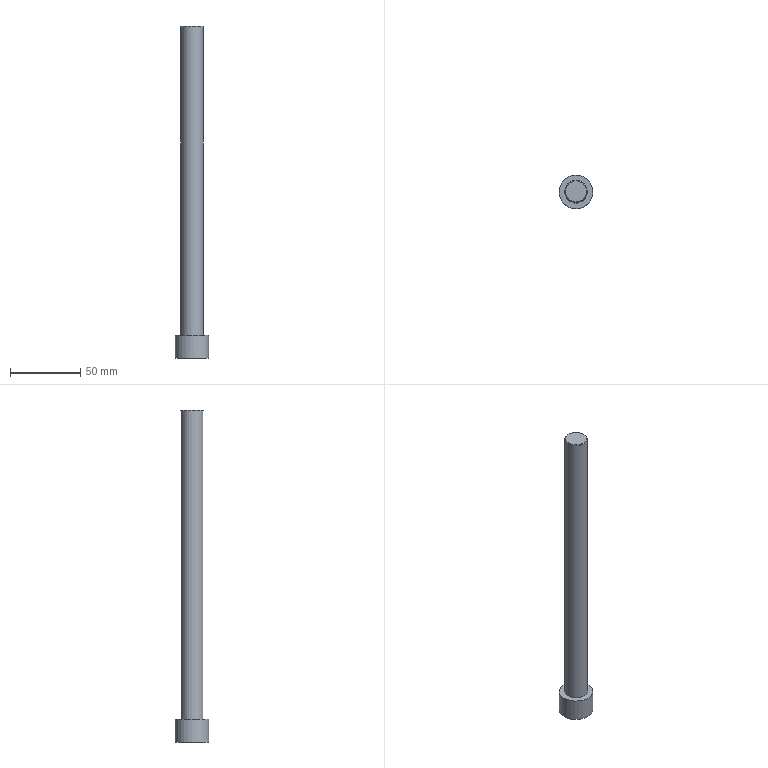Part | STEP file | 1_id586_xmt_txt | 1 solid | 19 faces | box 24 x 24 x 236 mm | volume 50039 mm3 | plane 15 | cylinder 2 | cone 2 | commonest cylinder face diameters 16 x1 24 x1
STEP:
#1=CARTESIAN_POINT('',(-153.,262.,-278.));
#2=VERTEX_POINT('',#1);
#3=CARTESIAN_POINT('',(-165.,262.,-278.));
#4=DIRECTION('',(0.,0.,-1.));
#5=DIRECTION('',(1.,0.,0.));
#6=AXIS2_PLACEMENT_3D('',#3,#4,#5);
#7=CIRCLE('',#6,12.);
#8=EDGE_CURVE('',#2,#2,#7,.T.);
#9=ORIENTED_EDGE('',*,*,#8,.F.);
#10=EDGE_LOOP('',(#9));
#11=FACE_BOUND('',#10,.T.);
#12=CARTESIAN_POINT('',(-153.,262.,-262.));
#13=VERTEX_POINT('',#12);
#14=CARTESIAN_POINT('',(-165.,262.,-262.));
#15=DIRECTION('',(0.,0.,1.));
#16=DIRECTION('',(1.,0.,0.));
#17=AXIS2_PLACEMENT_3D('',#14,#15,#16);
#18=CIRCLE('',#17,12.);
#19=EDGE_CURVE('',#13,#13,#18,.T.);
#20=ORIENTED_EDGE('',*,*,#19,.F.);
#21=EDGE_LOOP('',(#20));
#22=FACE_BOUND('',#21,.T.);
#23=CARTESIAN_POINT('',(-165.,262.,-270.));
#24=DIRECTION('',(0.,0.,1.));
#25=DIRECTION('',(-1.,0.,0.));
#26=AXIS2_PLACEMENT_3D('',#23,#24,#25);
#27=CYLINDRICAL_SURFACE('',#26,12.);
#28=ADVANCED_FACE('',(#11,#22),#27,.T.);
#29=CARTESIAN_POINT('',(-165.,270.083,-270.));
#30=VERTEX_POINT('',#29);
#31=CARTESIAN_POINT('',(-158.,266.041,-270.));
#32=VERTEX_POINT('',#31);
#33=CARTESIAN_POINT('',(-165.,262.,-270.));
#34=DIRECTION('',(0.,0.,-1.));
#35=DIRECTION('',(1.,0.,0.));
#36=AXIS2_PLACEMENT_3D('',#33,#34,#35);
#37=CIRCLE('',#36,8.083);
#38=EDGE_CURVE('',#30,#32,#37,.T.);
#39=ORIENTED_EDGE('',*,*,#38,.T.);
#40=CARTESIAN_POINT('',(-158.,257.959,-270.));
#41=VERTEX_POINT('',#40);
#42=CARTESIAN_POINT('',(-165.,262.,-270.));
#43=DIRECTION('',(0.,0.,-1.));
#44=DIRECTION('',(1.,0.,0.));
#45=AXIS2_PLACEMENT_3D('',#42,#43,#44);
#46=CIRCLE('',#45,8.083);
#47=EDGE_CURVE('',#32,#41,#46,.T.);
#48=ORIENTED_EDGE('',*,*,#47,.T.);
#49=CARTESIAN_POINT('',(-165.,253.917,-270.));
#50=VERTEX_POINT('',#49);
#51=CARTESIAN_POINT('',(-165.,262.,-270.));
#52=DIRECTION('',(0.,0.,-1.));
#53=DIRECTION('',(1.,0.,0.));
#54=AXIS2_PLACEMENT_3D('',#51,#52,#53);
#55=CIRCLE('',#54,8.083);
#56=EDGE_CURVE('',#41,#50,#55,.T.);
#57=ORIENTED_EDGE('',*,*,#56,.T.);
#58=CARTESIAN_POINT('',(-172.,257.959,-270.));
#59=VERTEX_POINT('',#58);
#60=CARTESIAN_POINT('',(-165.,262.,-270.));
#61=DIRECTION('',(0.,0.,-1.));
#62=DIRECTION('',(1.,0.,0.));
#63=AXIS2_PLACEMENT_3D('',#60,#61,#62);
#64=CIRCLE('',#63,8.083);
#65=EDGE_CURVE('',#50,#59,#64,.T.);
#66=ORIENTED_EDGE('',*,*,#65,.T.);
#67=CARTESIAN_POINT('',(-172.,266.041,-270.));
#68=VERTEX_POINT('',#67);
#69=CARTESIAN_POINT('',(-165.,262.,-270.));
#70=DIRECTION('',(0.,0.,-1.));
#71=DIRECTION('',(1.,0.,0.));
#72=AXIS2_PLACEMENT_3D('',#69,#70,#71);
#73=CIRCLE('',#72,8.083);
#74=EDGE_CURVE('',#59,#68,#73,.T.);
#75=ORIENTED_EDGE('',*,*,#74,.T.);
#76=CARTESIAN_POINT('',(-165.,262.,-270.));
#77=DIRECTION('',(0.,0.,-1.));
#78=DIRECTION('',(1.,0.,0.));
#79=AXIS2_PLACEMENT_3D('',#76,#77,#78);
#80=CIRCLE('',#79,8.083);
#81=EDGE_CURVE('',#68,#30,#80,.T.);
#82=ORIENTED_EDGE('',*,*,#81,.T.);
#83=EDGE_LOOP('',(#39,#48,#57,#66,#75,#82));
#84=FACE_BOUND('',#83,.T.);
#85=CARTESIAN_POINT('',(-165.,262.,-269.));
#86=VERTEX_POINT('',#85);
#87=VERTEX_LOOP('',#86);
#88=FACE_BOUND('',#87,.T.);
#89=CARTESIAN_POINT('',(-165.,262.,-269.5));
#90=DIRECTION('',(0.,0.,-1.));
#91=DIRECTION('',(-1.,0.,0.));
#92=AXIS2_PLACEMENT_3D('',#89,#90,#91);
#93=CONICAL_SURFACE('',#92,4.041,82.947);
#94=ADVANCED_FACE('',(#84,#88),#93,.F.);
#95=CARTESIAN_POINT('',(-157.,262.,-262.));
#96=VERTEX_POINT('',#95);
#97=CARTESIAN_POINT('',(-165.,262.,-262.));
#98=DIRECTION('',(0.,0.,-1.));
#99=DIRECTION('',(1.,0.,0.));
#100=AXIS2_PLACEMENT_3D('',#97,#98,#99);
#101=CIRCLE('',#100,8.);
#102=EDGE_CURVE('',#96,#96,#101,.T.);
#103=ORIENTED_EDGE('',*,*,#102,.F.);
#104=EDGE_LOOP('',(#103));
#105=FACE_BOUND('',#104,.T.);
#106=CARTESIAN_POINT('',(-173.,262.,-42.5));
#107=VERTEX_POINT('',#106);
#108=CARTESIAN_POINT('',(-165.,262.,-42.5));
#109=DIRECTION('',(0.,0.,1.));
#110=DIRECTION('',(-1.,0.,0.));
#111=AXIS2_PLACEMENT_3D('',#108,#109,#110);
#112=CIRCLE('',#111,8.);
#113=EDGE_CURVE('',#107,#107,#112,.T.);
#114=ORIENTED_EDGE('',*,*,#113,.F.);
#115=EDGE_LOOP('',(#114));
#116=FACE_BOUND('',#115,.T.);
#117=CARTESIAN_POINT('',(-165.,262.,-152.));
#118=DIRECTION('',(0.,0.,1.));
#119=DIRECTION('',(-1.,0.,0.));
#120=AXIS2_PLACEMENT_3D('',#117,#118,#119);
#121=CYLINDRICAL_SURFACE('',#120,8.);
#122=ADVANCED_FACE('',(#105,#116),#121,.T.);
#123=ORIENTED_EDGE('',*,*,#113,.T.);
#124=EDGE_LOOP('',(#123));
#125=FACE_BOUND('',#124,.T.);
#126=CARTESIAN_POINT('',(-172.5,262.,-42.));
#127=VERTEX_POINT('',#126);
#128=CARTESIAN_POINT('',(-165.,262.,-42.));
#129=DIRECTION('',(0.,0.,-1.));
#130=DIRECTION('',(-1.,0.,0.));
#131=AXIS2_PLACEMENT_3D('',#128,#129,#130);
#132=CIRCLE('',#131,7.5);
#133=EDGE_CURVE('',#127,#127,#132,.T.);
#134=ORIENTED_EDGE('',*,*,#133,.T.);
#135=EDGE_LOOP('',(#134));
#136=FACE_BOUND('',#135,.T.);
#137=CARTESIAN_POINT('',(-165.,262.,-42.));
#138=DIRECTION('',(0.,0.,-1.));
#139=DIRECTION('',(1.,0.,0.));
#140=AXIS2_PLACEMENT_3D('',#137,#138,#139);
#141=CONICAL_SURFACE('',#140,7.5,45.);
#142=ADVANCED_FACE('',(#125,#136),#141,.T.);
#143=ORIENTED_EDGE('',*,*,#133,.F.);
#144=EDGE_LOOP('',(#143));
#145=FACE_OUTER_BOUND('',#144,.T.);
#146=CARTESIAN_POINT('',(-165.,262.,-42.));
#147=DIRECTION('',(0.,0.,1.));
#148=DIRECTION('',(-1.,0.,0.));
#149=AXIS2_PLACEMENT_3D('',#146,#147,#148);
#150=PLANE('',#149);
#151=ADVANCED_FACE('',(#145),#150,.T.);
#152=CARTESIAN_POINT('',(-161.5,255.938,-270.));
#153=DIRECTION('',(0.866,0.5,0.));
#154=VECTOR('',#153,1.);
#155=LINE('',#152,#154);
#156=EDGE_CURVE('',#50,#41,#155,.T.);
#157=ORIENTED_EDGE('',*,*,#156,.F.);
#158=ORIENTED_EDGE('',*,*,#56,.F.);
#159=EDGE_LOOP('',(#157,#158));
#160=FACE_OUTER_BOUND('',#159,.T.);
#161=CARTESIAN_POINT('',(-165.,262.,-270.));
#162=DIRECTION('',(0.,0.,-1.));
#163=DIRECTION('',(1.,0.,0.));
#164=AXIS2_PLACEMENT_3D('',#161,#162,#163);
#165=PLANE('',#164);
#166=ADVANCED_FACE('',(#160),#165,.F.);
#167=CARTESIAN_POINT('',(-158.,262.,-270.));
#168=DIRECTION('',(0.,1.,0.));
#169=VECTOR('',#168,1.);
#170=LINE('',#167,#169);
#171=EDGE_CURVE('',#41,#32,#170,.T.);
#172=ORIENTED_EDGE('',*,*,#171,.F.);
#173=ORIENTED_EDGE('',*,*,#47,.F.);
#174=EDGE_LOOP('',(#172,#173));
#175=FACE_OUTER_BOUND('',#174,.T.);
#176=CARTESIAN_POINT('',(-165.,262.,-270.));
#177=DIRECTION('',(0.,0.,-1.));
#178=DIRECTION('',(1.,0.,0.));
#179=AXIS2_PLACEMENT_3D('',#176,#177,#178);
#180=PLANE('',#179);
#181=ADVANCED_FACE('',(#175),#180,.F.);
#182=CARTESIAN_POINT('',(-161.5,268.062,-270.));
#183=DIRECTION('',(-0.866,0.5,0.));
#184=VECTOR('',#183,1.);
#185=LINE('',#182,#184);
#186=EDGE_CURVE('',#32,#30,#185,.T.);
#187=ORIENTED_EDGE('',*,*,#186,.F.);
#188=ORIENTED_EDGE('',*,*,#38,.F.);
#189=EDGE_LOOP('',(#187,#188));
#190=FACE_OUTER_BOUND('',#189,.T.);
#191=CARTESIAN_POINT('',(-165.,262.,-270.));
#192=DIRECTION('',(0.,0.,-1.));
#193=DIRECTION('',(1.,0.,0.));
#194=AXIS2_PLACEMENT_3D('',#191,#192,#193);
#195=PLANE('',#194);
#196=ADVANCED_FACE('',(#190),#195,.F.);
#197=CARTESIAN_POINT('',(-168.5,268.062,-270.));
#198=DIRECTION('',(-0.866,-0.5,0.));
#199=VECTOR('',#198,1.);
#200=LINE('',#197,#199);
#201=EDGE_CURVE('',#30,#68,#200,.T.);
#202=ORIENTED_EDGE('',*,*,#201,.F.);
#203=ORIENTED_EDGE('',*,*,#81,.F.);
#204=EDGE_LOOP('',(#202,#203));
#205=FACE_OUTER_BOUND('',#204,.T.);
#206=CARTESIAN_POINT('',(-165.,262.,-270.));
#207=DIRECTION('',(0.,0.,-1.));
#208=DIRECTION('',(1.,0.,0.));
#209=AXIS2_PLACEMENT_3D('',#206,#207,#208);
#210=PLANE('',#209);
#211=ADVANCED_FACE('',(#205),#210,.F.);
#212=CARTESIAN_POINT('',(-172.,262.,-270.));
#213=DIRECTION('',(0.,-1.,0.));
#214=VECTOR('',#213,1.);
#215=LINE('',#212,#214);
#216=EDGE_CURVE('',#68,#59,#215,.T.);
#217=ORIENTED_EDGE('',*,*,#216,.F.);
#218=ORIENTED_EDGE('',*,*,#74,.F.);
#219=EDGE_LOOP('',(#217,#218));
#220=FACE_OUTER_BOUND('',#219,.T.);
#221=CARTESIAN_POINT('',(-165.,262.,-270.));
#222=DIRECTION('',(0.,0.,-1.));
#223=DIRECTION('',(1.,0.,0.));
#224=AXIS2_PLACEMENT_3D('',#221,#222,#223);
#225=PLANE('',#224);
#226=ADVANCED_FACE('',(#220),#225,.F.);
#227=CARTESIAN_POINT('',(-168.5,255.938,-270.));
#228=DIRECTION('',(0.866,-0.5,0.));
#229=VECTOR('',#228,1.);
#230=LINE('',#227,#229);
#231=EDGE_CURVE('',#59,#50,#230,.T.);
#232=ORIENTED_EDGE('',*,*,#231,.F.);
#233=ORIENTED_EDGE('',*,*,#65,.F.);
#234=EDGE_LOOP('',(#232,#233));
#235=FACE_OUTER_BOUND('',#234,.T.);
#236=CARTESIAN_POINT('',(-165.,262.,-270.));
#237=DIRECTION('',(0.,0.,-1.));
#238=DIRECTION('',(1.,0.,0.));
#239=AXIS2_PLACEMENT_3D('',#236,#237,#238);
#240=PLANE('',#239);
#241=ADVANCED_FACE('',(#235),#240,.F.);
#242=CARTESIAN_POINT('',(-165.,253.917,-278.));
#243=VERTEX_POINT('',#242);
#244=CARTESIAN_POINT('',(-165.,253.917,-274.));
#245=DIRECTION('',(0.,0.,-1.));
#246=VECTOR('',#245,1.);
#247=LINE('',#244,#246);
#248=EDGE_CURVE('',#50,#243,#247,.T.);
#249=ORIENTED_EDGE('',*,*,#248,.F.);
#250=ORIENTED_EDGE('',*,*,#156,.T.);
#251=CARTESIAN_POINT('',(-158.,257.959,-278.));
#252=VERTEX_POINT('',#251);
#253=CARTESIAN_POINT('',(-158.,257.959,-274.));
#254=DIRECTION('',(0.,0.,-1.));
#255=VECTOR('',#254,1.);
#256=LINE('',#253,#255);
#257=EDGE_CURVE('',#41,#252,#256,.T.);
#258=ORIENTED_EDGE('',*,*,#257,.T.);
#259=CARTESIAN_POINT('',(-161.5,255.938,-278.));
#260=DIRECTION('',(0.866,0.5,0.));
#261=VECTOR('',#260,1.);
#262=LINE('',#259,#261);
#263=EDGE_CURVE('',#243,#252,#262,.T.);
#264=ORIENTED_EDGE('',*,*,#263,.F.);
#265=EDGE_LOOP('',(#249,#250,#258,#264));
#266=FACE_OUTER_BOUND('',#265,.T.);
#267=CARTESIAN_POINT('',(-161.5,255.938,-274.));
#268=DIRECTION('',(-0.5,0.866,0.));
#269=DIRECTION('',(0.,0.,-1.));
#270=AXIS2_PLACEMENT_3D('',#267,#268,#269);
#271=PLANE('',#270);
#272=ADVANCED_FACE('',(#266),#271,.T.);
#273=CARTESIAN_POINT('',(-172.,257.959,-278.));
#274=VERTEX_POINT('',#273);
#275=CARTESIAN_POINT('',(-172.,257.959,-274.));
#276=DIRECTION('',(0.,0.,-1.));
#277=VECTOR('',#276,1.);
#278=LINE('',#275,#277);
#279=EDGE_CURVE('',#59,#274,#278,.T.);
#280=ORIENTED_EDGE('',*,*,#279,.F.);
#281=ORIENTED_EDGE('',*,*,#231,.T.);
#282=ORIENTED_EDGE('',*,*,#248,.T.);
#283=CARTESIAN_POINT('',(-168.5,255.938,-278.));
#284=DIRECTION('',(0.866,-0.5,0.));
#285=VECTOR('',#284,1.);
#286=LINE('',#283,#285);
#287=EDGE_CURVE('',#274,#243,#286,.T.);
#288=ORIENTED_EDGE('',*,*,#287,.F.);
#289=EDGE_LOOP('',(#280,#281,#282,#288));
#290=FACE_OUTER_BOUND('',#289,.T.);
#291=CARTESIAN_POINT('',(-168.5,255.938,-274.));
#292=DIRECTION('',(0.5,0.866,0.));
#293=DIRECTION('',(0.,0.,1.));
#294=AXIS2_PLACEMENT_3D('',#291,#292,#293);
#295=PLANE('',#294);
#296=ADVANCED_FACE('',(#290),#295,.T.);
#297=CARTESIAN_POINT('',(-172.,266.041,-278.));
#298=VERTEX_POINT('',#297);
#299=CARTESIAN_POINT('',(-172.,266.041,-274.));
#300=DIRECTION('',(0.,0.,-1.));
#301=VECTOR('',#300,1.);
#302=LINE('',#299,#301);
#303=EDGE_CURVE('',#68,#298,#302,.T.);
#304=ORIENTED_EDGE('',*,*,#303,.F.);
#305=ORIENTED_EDGE('',*,*,#216,.T.);
#306=ORIENTED_EDGE('',*,*,#279,.T.);
#307=CARTESIAN_POINT('',(-172.,262.,-278.));
#308=DIRECTION('',(0.,-1.,0.));
#309=VECTOR('',#308,1.);
#310=LINE('',#307,#309);
#311=EDGE_CURVE('',#298,#274,#310,.T.);
#312=ORIENTED_EDGE('',*,*,#311,.F.);
#313=EDGE_LOOP('',(#304,#305,#306,#312));
#314=FACE_OUTER_BOUND('',#313,.T.);
#315=CARTESIAN_POINT('',(-172.,262.,-274.));
#316=DIRECTION('',(1.,0.,0.));
#317=DIRECTION('',(0.,0.,1.));
#318=AXIS2_PLACEMENT_3D('',#315,#316,#317);
#319=PLANE('',#318);
#320=ADVANCED_FACE('',(#314),#319,.T.);
#321=CARTESIAN_POINT('',(-165.,270.083,-278.));
#322=VERTEX_POINT('',#321);
#323=CARTESIAN_POINT('',(-165.,270.083,-274.));
#324=DIRECTION('',(0.,0.,-1.));
#325=VECTOR('',#324,1.);
#326=LINE('',#323,#325);
#327=EDGE_CURVE('',#30,#322,#326,.T.);
#328=ORIENTED_EDGE('',*,*,#327,.F.);
#329=ORIENTED_EDGE('',*,*,#201,.T.);
#330=ORIENTED_EDGE('',*,*,#303,.T.);
#331=CARTESIAN_POINT('',(-168.5,268.062,-278.));
#332=DIRECTION('',(-0.866,-0.5,0.));
#333=VECTOR('',#332,1.);
#334=LINE('',#331,#333);
#335=EDGE_CURVE('',#322,#298,#334,.T.);
#336=ORIENTED_EDGE('',*,*,#335,.F.);
#337=EDGE_LOOP('',(#328,#329,#330,#336));
#338=FACE_OUTER_BOUND('',#337,.T.);
#339=CARTESIAN_POINT('',(-168.5,268.062,-274.));
#340=DIRECTION('',(0.5,-0.866,0.));
#341=DIRECTION('',(0.,0.,1.));
#342=AXIS2_PLACEMENT_3D('',#339,#340,#341);
#343=PLANE('',#342);
#344=ADVANCED_FACE('',(#338),#343,.T.);
#345=CARTESIAN_POINT('',(-158.,266.041,-278.));
#346=VERTEX_POINT('',#345);
#347=CARTESIAN_POINT('',(-158.,266.041,-274.));
#348=DIRECTION('',(0.,0.,-1.));
#349=VECTOR('',#348,1.);
#350=LINE('',#347,#349);
#351=EDGE_CURVE('',#32,#346,#350,.T.);
#352=ORIENTED_EDGE('',*,*,#351,.F.);
#353=ORIENTED_EDGE('',*,*,#186,.T.);
#354=ORIENTED_EDGE('',*,*,#327,.T.);
#355=CARTESIAN_POINT('',(-161.5,268.062,-278.));
#356=DIRECTION('',(-0.866,0.5,0.));
#357=VECTOR('',#356,1.);
#358=LINE('',#355,#357);
#359=EDGE_CURVE('',#346,#322,#358,.T.);
#360=ORIENTED_EDGE('',*,*,#359,.F.);
#361=EDGE_LOOP('',(#352,#353,#354,#360));
#362=FACE_OUTER_BOUND('',#361,.T.);
#363=CARTESIAN_POINT('',(-161.5,268.062,-274.));
#364=DIRECTION('',(-0.5,-0.866,0.));
#365=DIRECTION('',(0.,0.,-1.));
#366=AXIS2_PLACEMENT_3D('',#363,#364,#365);
#367=PLANE('',#366);
#368=ADVANCED_FACE('',(#362),#367,.T.);
#369=ORIENTED_EDGE('',*,*,#257,.F.);
#370=ORIENTED_EDGE('',*,*,#171,.T.);
#371=ORIENTED_EDGE('',*,*,#351,.T.);
#372=CARTESIAN_POINT('',(-158.,262.,-278.));
#373=DIRECTION('',(0.,1.,0.));
#374=VECTOR('',#373,1.);
#375=LINE('',#372,#374);
#376=EDGE_CURVE('',#252,#346,#375,.T.);
#377=ORIENTED_EDGE('',*,*,#376,.F.);
#378=EDGE_LOOP('',(#369,#370,#371,#377));
#379=FACE_OUTER_BOUND('',#378,.T.);
#380=CARTESIAN_POINT('',(-158.,262.,-274.));
#381=DIRECTION('',(-1.,0.,0.));
#382=DIRECTION('',(0.,0.,-1.));
#383=AXIS2_PLACEMENT_3D('',#380,#381,#382);
#384=PLANE('',#383);
#385=ADVANCED_FACE('',(#379),#384,.T.);
#386=ORIENTED_EDGE('',*,*,#263,.T.);
#387=ORIENTED_EDGE('',*,*,#376,.T.);
#388=ORIENTED_EDGE('',*,*,#359,.T.);
#389=ORIENTED_EDGE('',*,*,#335,.T.);
#390=ORIENTED_EDGE('',*,*,#311,.T.);
#391=ORIENTED_EDGE('',*,*,#287,.T.);
#392=EDGE_LOOP('',(#386,#387,#388,#389,#390,#391));
#393=FACE_BOUND('',#392,.T.);
#394=ORIENTED_EDGE('',*,*,#8,.T.);
#395=EDGE_LOOP('',(#394));
#396=FACE_BOUND('',#395,.T.);
#397=CARTESIAN_POINT('',(-165.,262.,-278.));
#398=DIRECTION('',(0.,0.,-1.));
#399=DIRECTION('',(1.,0.,0.));
#400=AXIS2_PLACEMENT_3D('',#397,#398,#399);
#401=PLANE('',#400);
#402=ADVANCED_FACE('',(#393,#396),#401,.T.);
#403=ORIENTED_EDGE('',*,*,#102,.T.);
#404=EDGE_LOOP('',(#403));
#405=FACE_BOUND('',#404,.T.);
#406=ORIENTED_EDGE('',*,*,#19,.T.);
#407=EDGE_LOOP('',(#406));
#408=FACE_BOUND('',#407,.T.);
#409=CARTESIAN_POINT('',(-165.,262.,-262.));
#410=DIRECTION('',(0.,0.,1.));
#411=DIRECTION('',(-1.,0.,0.));
#412=AXIS2_PLACEMENT_3D('',#409,#410,#411);
#413=PLANE('',#412);
#414=ADVANCED_FACE('',(#405,#408),#413,.T.);
#415=CLOSED_SHELL('',(#28,#94,#122,#142,#151,#166,#181,#196,#211,#226,#241,#272,#296,#320,#344,#368,#385,#402,#414));
#416=MANIFOLD_SOLID_BREP('',#415);
#417=(LENGTH_UNIT()NAMED_UNIT(*)SI_UNIT(.MILLI.,.METRE.));
#418=UNCERTAINTY_MEASURE_WITH_UNIT(LENGTH_MEASURE(0.00002),#417,'','');
#419=(NAMED_UNIT(*)PLANE_ANGLE_UNIT()SI_UNIT($,.RADIAN.));
#420=PLANE_ANGLE_MEASURE_WITH_UNIT(PLANE_ANGLE_MEASURE(0.01745),#419);
#421=DIMENSIONAL_EXPONENTS(0.,0.,0.,0.,0.,0.,0.);
#422=(CONVERSION_BASED_UNIT('DEGREE',#420)NAMED_UNIT(#421)PLANE_ANGLE_UNIT());
#423=(NAMED_UNIT(*)SI_UNIT($,.STERADIAN.)SOLID_ANGLE_UNIT());
#424=(GEOMETRIC_REPRESENTATION_CONTEXT(3)GLOBAL_UNCERTAINTY_ASSIGNED_CONTEXT((#418))GLOBAL_UNIT_ASSIGNED_CONTEXT((#417,#422,#423))REPRESENTATION_CONTEXT('',''));
#425=ADVANCED_BREP_SHAPE_REPRESENTATION('',(#416),#424);